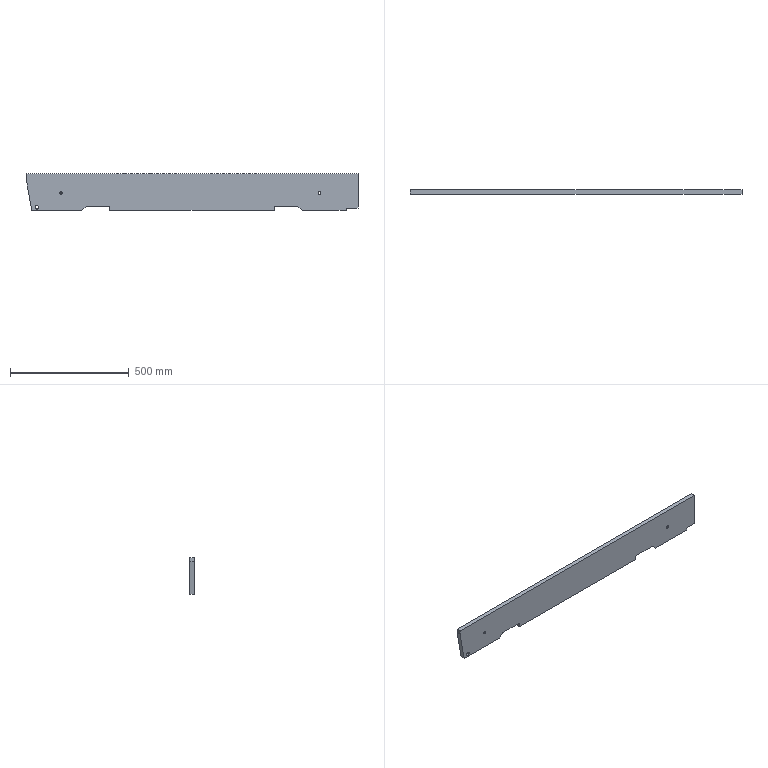Part | STEP file | Frame_right | 1 solid | 20 faces | box 1400 x 18 x 155 mm | volume 3789981 mm3 | plane 17 | cylinder 3 | commonest cylinder face diameters 11 x2 15 x1